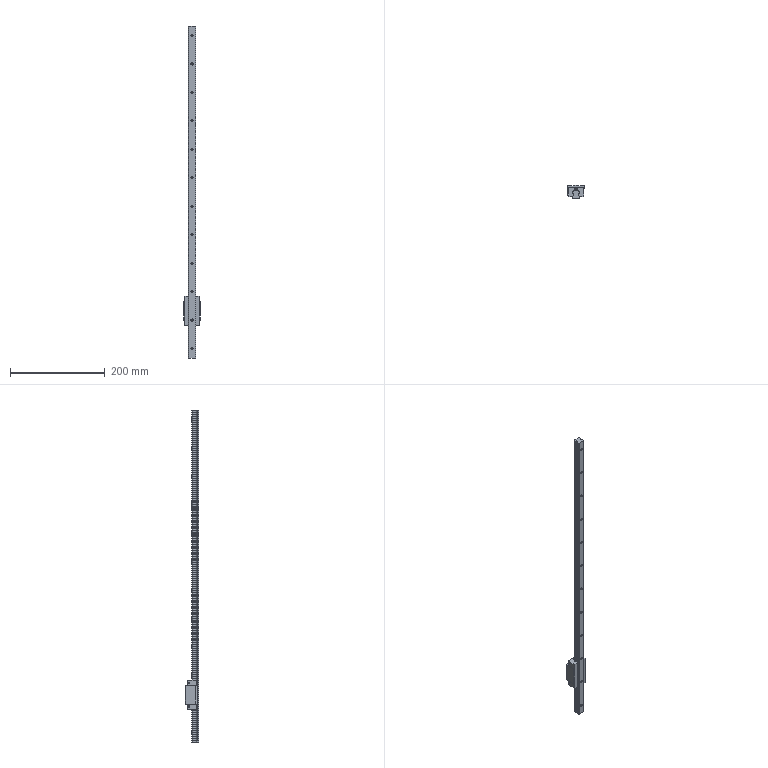Part | SolidWorks | 2 solids | 209 faces | box 34 x 28 x 700 mm | volume 165432 mm3 | cylinder 107 | plane 102 | commonest cylinder face diameters 4.5 x24 7.5 x24 0.8 x16 4 x13 3.24 x8 3.3 x8